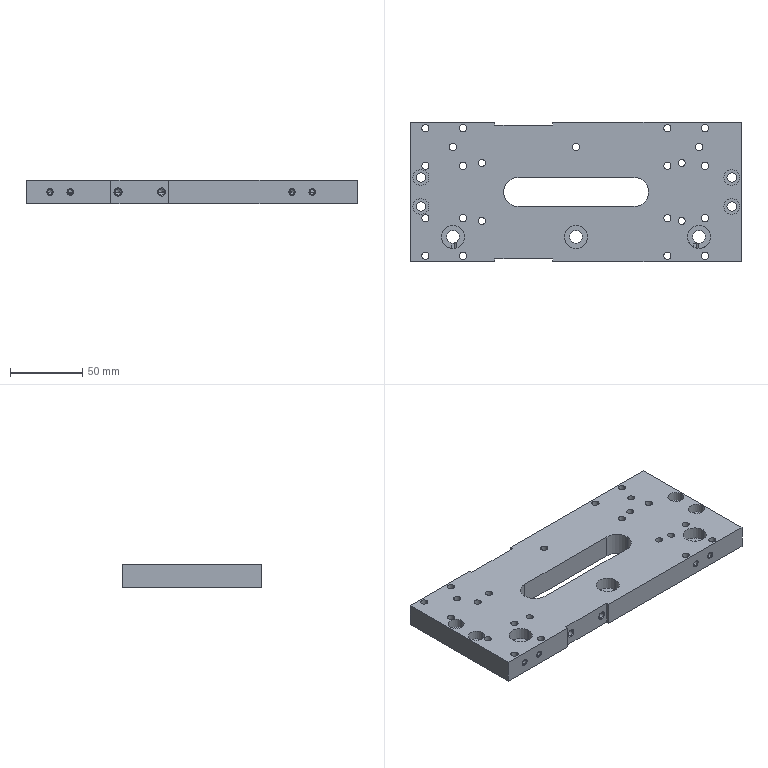Part | NX | 1 solid | 188 faces | box 228 x 96 x 16 mm | volume 297749 mm3 | cylinder 105 | cone 60 | plane 23 | commonest cylinder face diameters 5 x46 3.3 x16 4.2 x8 6.6 x8 11 x8 8.8 x6